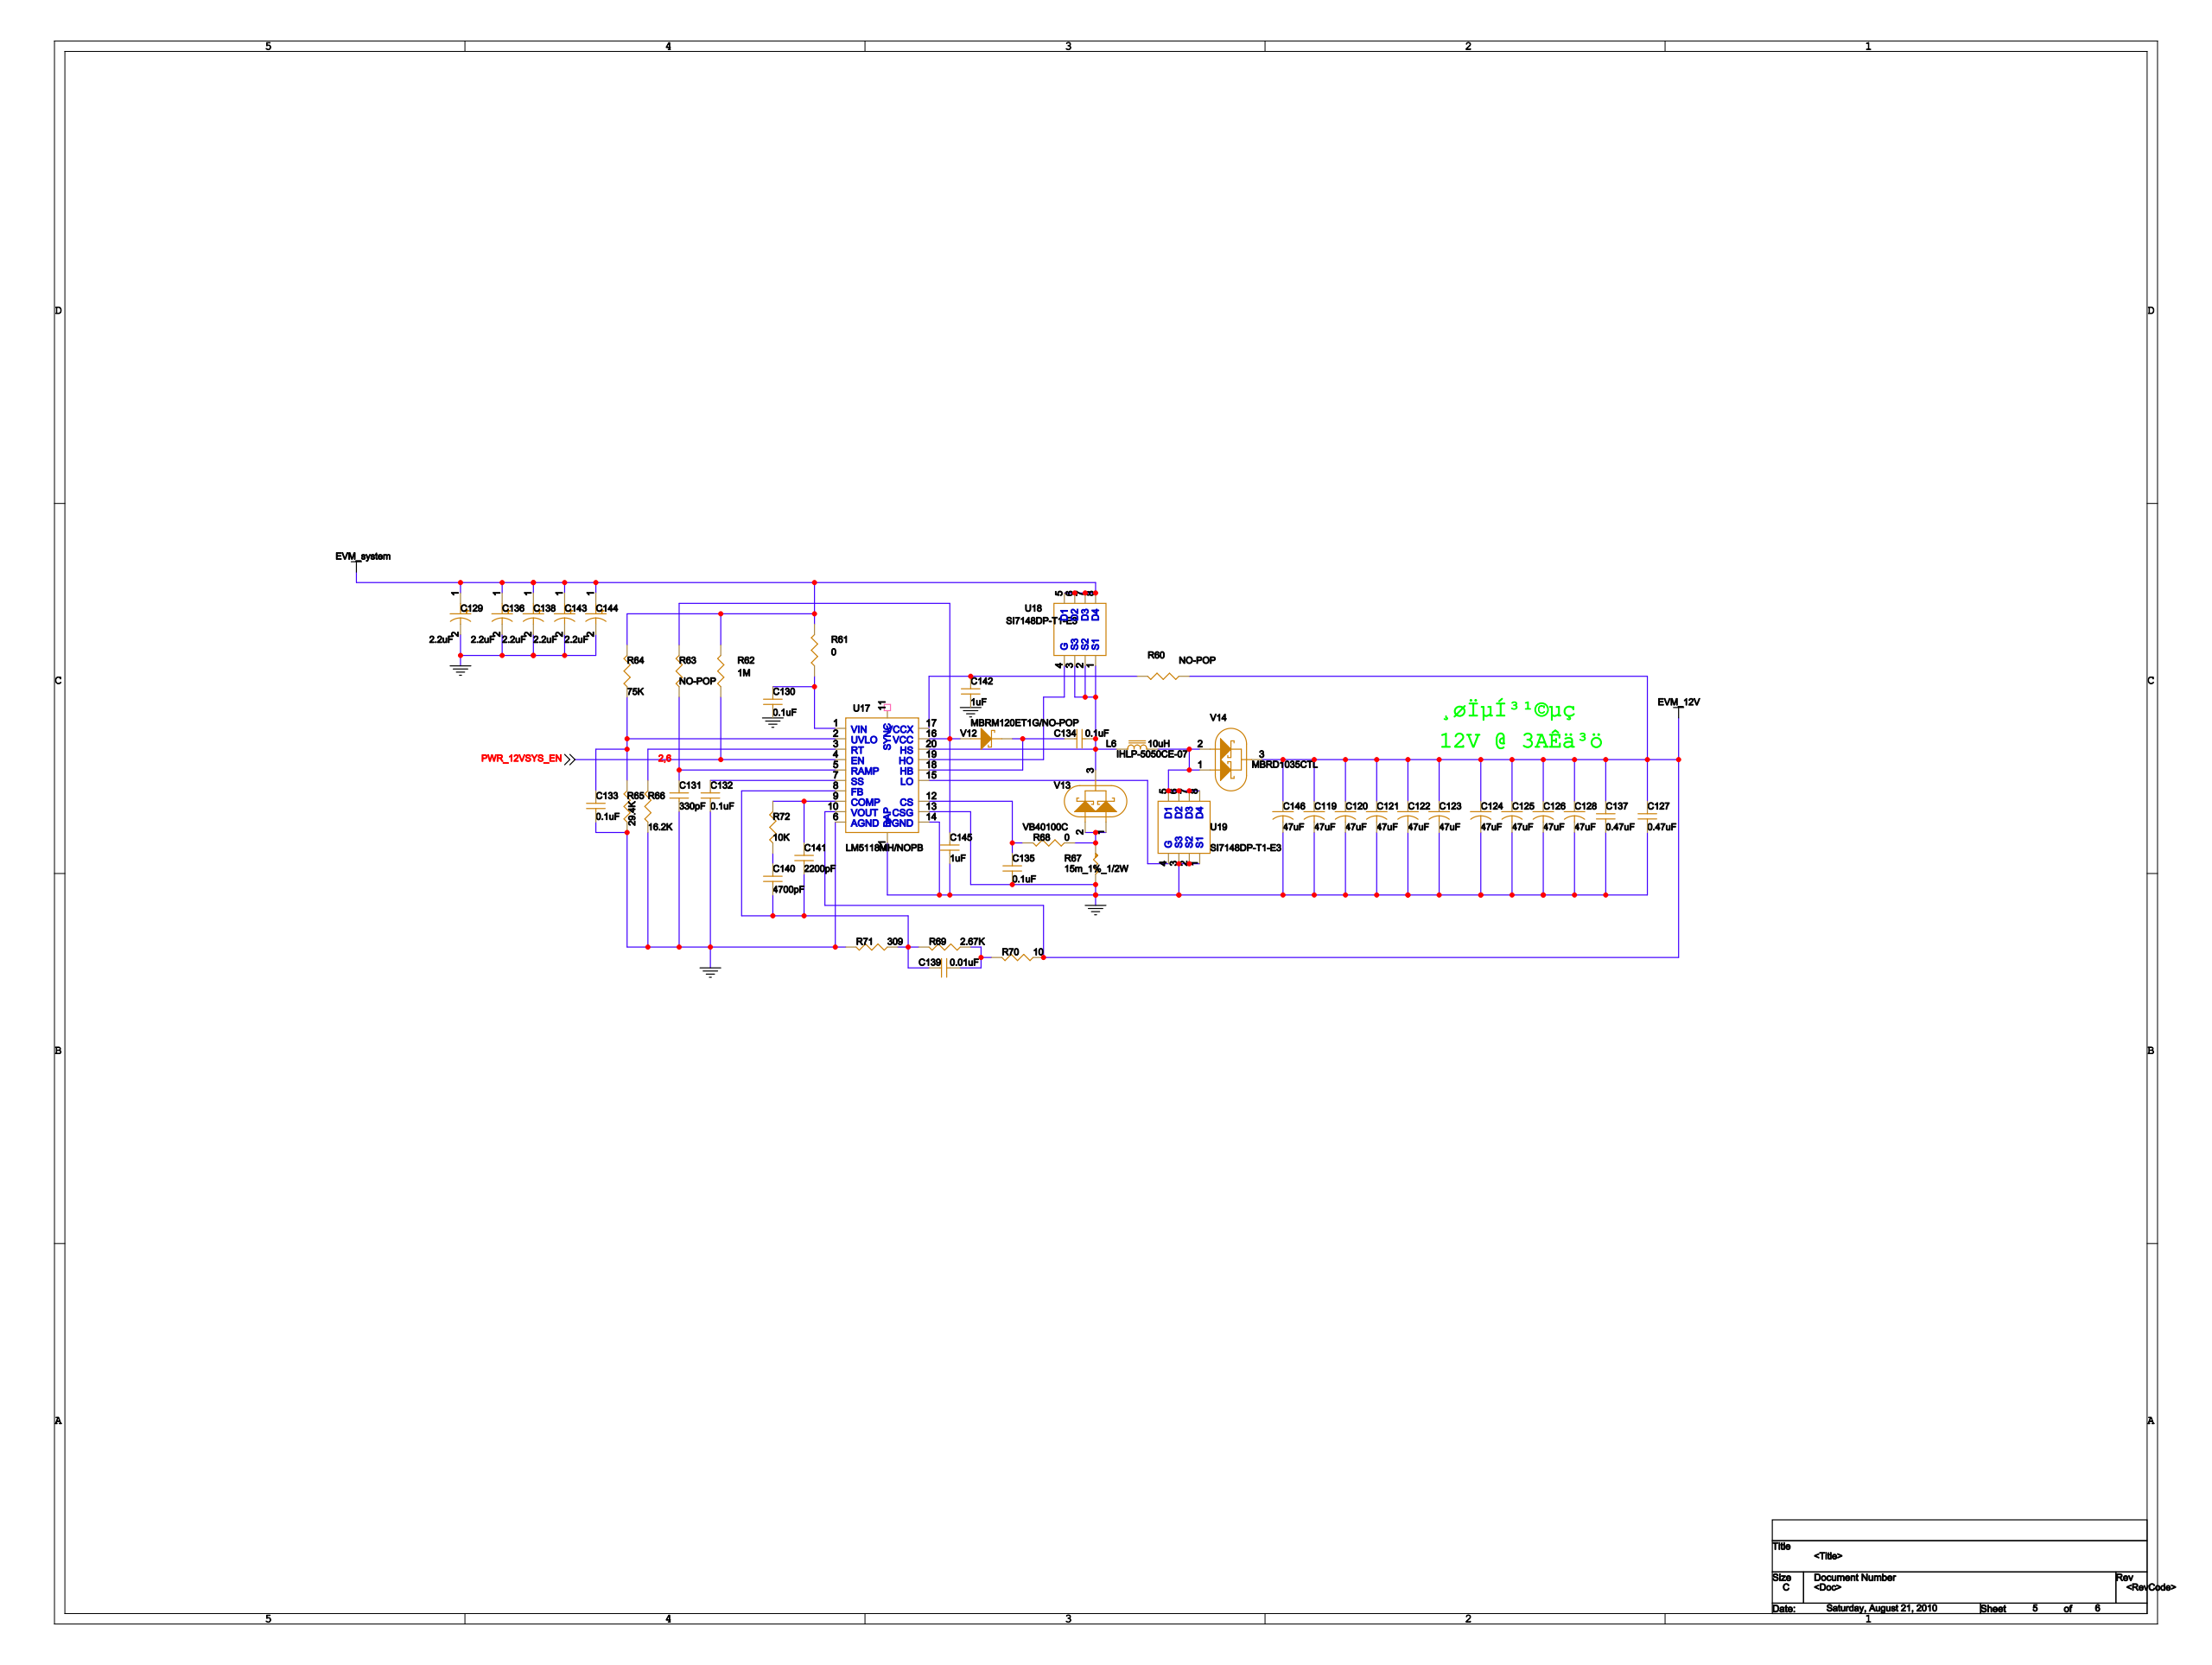Circuit board | Cadence Allegro | 241 parts | 116 nets | one sheet of the schematic
Parts on this sheet (reference | value | footprint):
C119 | 47uF | C1210
C120 | 47uF | C1210
C121 | 47uF | C1210
C122 | 47uF | C1210
C123 | 47uF | C1210
C124 | 47uF | C1210
C125 | 47uF | C1210
C126 | 47uF | C1210
C129 | 22uF | C1210
C130 | 0.1uF | R0603
C131 | 330pF | C0603
C132 | 0.1uF | C0603
C133 | 0.1uF | R0603
C134 | 0.1uF | C0603
C135 | 0.1uF | C0603
C139 | 0.01uF | C0603
C140 | 4700pF | C0603
C141 | 2200pF | C0603
C142 | 1uF | C0603
C145 | 1uF | C0603
C146 | 47uF | C1210
L6 | 10uH | L-12X12X7
R60 | NO-POP | R0603
R61 | 0 | R0603
R62 | 1M | R0603
R63 | NO-POP | R0603
R64 | 75K | R0603
R66 | 16.2K | R0603
R67 | 15m_1%_1/2W | R1206
R68 | 0 | R0603
R69 | 2.67K | R0603
R70 | 10 | R0603
R71 | 309 | R0603
R72 | 10K | R0603
U17 | LM5118MH/NOPB | TSSOP-20EP
U18 | SI7148DP-T1-E3 | SO_8_PAD
U19 | SI7148DP-T1-E3 | SO_8_PAD
V12 | MBRM120ET1G | DO_216AA
V13 | MBRD1035CTL | TO-263AB
V14 | MBRD1035CTL | TO-252-2
Nets of these parts (net: part-pin ...):
EVM_SYSTEM: C129-1 R61-2 R62-2 R64-2 U18-5 U18-6 U18-7 U18-8
GND: C119-2 C120-2 C121-2 C122-2 C123-2 C124-2 C125-2 C126-2 C129-2 C130-2 C131-2 C132-2 C133-2 C135-2 C142-2 C145-2 C146-2 R66-1 R67-2 R71-2 U17-6 U17-13 U17-14 U17-21 U19-1 U19-2 U19-3
N19248210: C132-1 U17-7
N19248308: C134-1 U17-18 V12-1
N19248288: C134-2 L6-1 U17-20 U18-1 U18-2 U18-3 V13-3
N19248384: C135-1 R68-2 U17-12
N19248126: C130-1 R61-1 U17-1
N19248220: C133-1 R64-1 U17-2
EVM_12V: C119-1 C120-1 C121-1 C122-1 C123-1 C124-1 C125-1 C126-1 C146-1 R60-1 R70-1 U17-10 V14-3
N19248186: C131-1 R63-1 U17-5
N19248561: C139-1 C140-2 C141-2 R69-2 R71-1 U17-8
N19248015: C139-2 R69-1 R70-2
N19248013: C140-1 R72-1
N19248615: C141-1 R72-2 U17-9
N19248411: L6-2 U19-5 U19-6 U19-7 U19-8 V14-1 V14-2
N19248349: R67-1 R68-1 V13-1 V13-2
N19248049: C142-1 R60-2 U17-17
N19248256: C145-1 R63-2 U17-16 V12-2
N19247881: R62-1 U17-4
N19248226: R66-2 U17-3
N19248328: U17-19 U18-4
N19248451: U17-15 U19-4